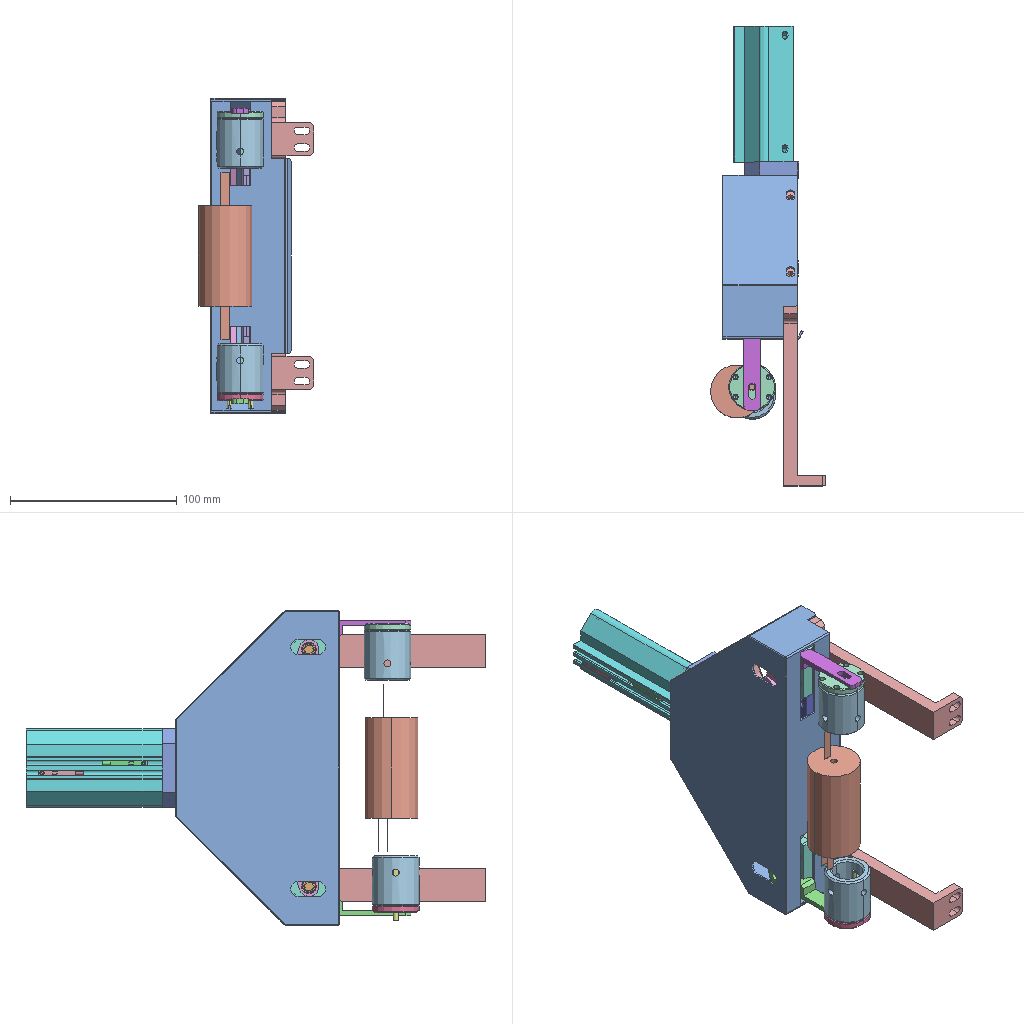Assembly | SolidWorks | 26 different items | 33 placed | box 69 x 276 x 189 mm
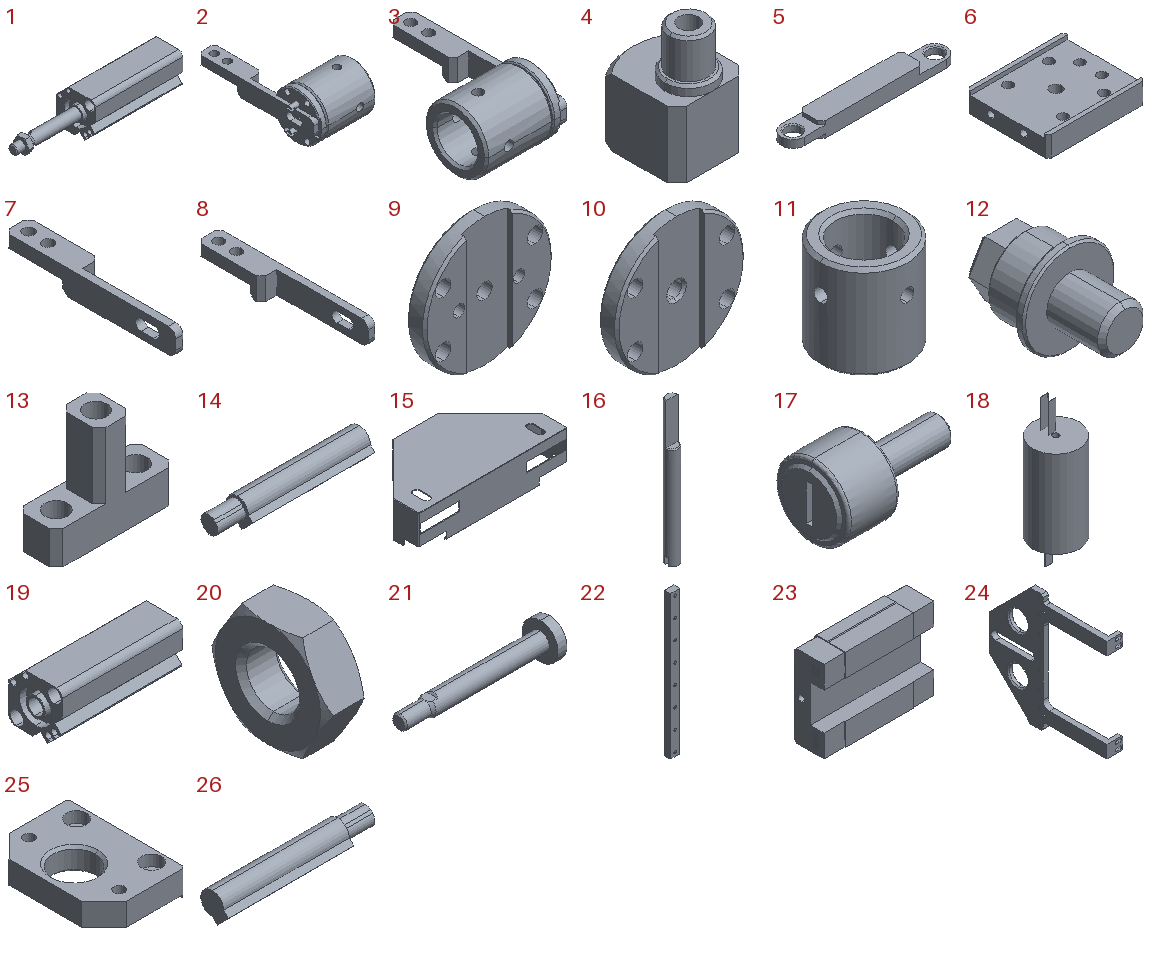Parts list (item | name | quantity | parent item | size | volume | features):
1 | (subassembly) | x1 | - | 140.657 x 36 x 36 mm | 68921 mm3 | features AEMSimFeature 1
2 | (subassembly) | x1 | - | 39 x 72.074 x 28 mm | 15051 mm3 | -
3 | (subassembly) | x1 | - | 36 x 70 x 28 mm | 14685 mm3 | -
4 | - | x1 | - | 15 x 17.5 x 24 mm | 3225 mm3 | features Chamfer 3, ICE 3, HoleWzd 2, Extrusion 1
5 | - | x2 | - | 87 x 12 x 8 mm | 6197 mm3 | features Chamfer 2, ICE 2, Extrusion 1
6 | - | x2 | - | 35.5 x 30 x 10.5 mm | 5956 mm3 | features HoleWzd 4, Chamfer 3, Cut 1, Extrusion 1, ICE 1
7 | - | x1 | in 2 | 10 x 70 x 10 mm | 2584 mm3 | features ICE 3, Chamfer 1, Extrusion 1, Fillet 1, HoleWzd 1
8 | - | x1 | in 3 | 10 x 70 x 10 mm | 2584 mm3 | features ICE 3, Chamfer 1, Extrusion 1, Fillet 1, HoleWzd 1
9 | - | x1 | in 2 | 28 x 5 x 28 mm | 2209 mm3 | features HoleWzd 3, Chamfer 2, ICE 2, Revolution 1
10 | - | x1 | in 3 | 28 x 5 x 28 mm | 2255 mm3 | features Chamfer 2, HoleWzd 2, ICE 2, Revolution 1
11 | - | x2 | in 2, 3 | 28 x 28 x 30 mm | 9846 mm3 | features HoleWzd 5, Chamfer 1, Extrusion 1
12 | - | x2 | - | 10 x 14 x 10 mm | 484.922 mm3 | features Chamfer 2, ICE 1, Revolution 1
13 | - | x2 | - | 18 x 6 x 15 mm | 590.913 mm3 | features Chamfer 2, HoleWzd 2, Extrusion 1, ICE 1
14 | - | x1 | in 1 | 27 x 4.828 x 4.828 mm | 354.995 mm3 | features BaseBody 1
15 | - | x1 | - | 189 x 98 x 48.5 mm | 32493 mm3 | features ICE 5, Chamfer 2, Fillet 2, BossThin 1, FlatPattern 1, MirrorPattern 1, SMBaseFlange 1, SheetMetal 1, Shell 1
16 | - | x2 | in 2 | 3 x 3 x 35 mm | 205.851 mm3 | features ICE 2, Chamfer 1, Extrusion 1
17 | - | x1 | - | 23 x 13 x 13 mm | 1507 mm3 | features ICE 1, Revolution 1
18 | - | x1 | - | 32 x 32 x 100 mm | 47531 mm3 | features ICE 2, Extrusion 1
19 | - | x1 | in 1 | 81.5 x 36 x 36 mm | 60391 mm3 | features BaseBody 1
20 | - | x1 | in 1 | 5 x 15.011 x 13 mm | 543.249 mm3 | features BaseBody 1
21 | - | x1 | in 1 | 83.5 x 20 x 20 mm | 7277 mm3 | features BaseBody 1
22 | - | x1 | - | 12 x 7.5 x 185 mm | 15537 mm3 | features Chamfer 1, Extrusion 1, HoleWzd 1, LPattern 1
23 | - | x2 | - | 35.4 x 10 x 27 mm | 7144 mm3 | features ICE 49, Chamfer 34, HoleWzd 16, RevCut 4, BaseBody 1
24 | - | x1 | - | 25 x 185 x 185 mm | 107483 mm3 | features HoleWzd 4, ICE 4, Chamfer 3, Fillet 2, Extrusion 1, MirrorPattern 1
25 | - | x1 | - | 32.5 x 47 x 10 mm | 10119 mm3 | features Chamfer 2, HoleWzd 2, ICE 2, Extrusion 1
26 | - | x1 | in 1 | 27 x 4.828 x 4.828 mm | 354.995 mm3 | features BaseBody 1
Mates (type | each side: item.copy, entity, surface, feature):
In the top assembly
DistanceDim | 18.1 plane | 24.1 face plane Boss-Extrude1
Coincident | 24.1 face plane Boss-Extrude1 | 22.1 face plane Boss-Extrude1
Width | 24.1 face plane Boss-Extrude1 | 24.1 face plane Boss-Extrude1 | 22.1 face plane Boss-Extrude1 | 22.1 face plane Boss-Extrude1
Coincident | 22.1 face plane Boss-Extrude1 | 23.1 face plane Cut-Revolve1
Coincident | 22.1 face plane Boss-Extrude1 | 23.2 face plane Cut-Revolve1
Coincident | 23.2 face plane Cut-Extrude41 | 22.1 face plane Boss-Extrude1
Coincident | 22.1 face plane Boss-Extrude1 | 23.1 face plane Cut-Extrude41
DistanceDim | 22.1 face plane Boss-Extrude1 | 24.1 face plane Boss-Extrude1
Coincident | 23.1 face plane Input3 | 6.1 face plane Cut-Extrude1
Coincident | 23.1 face plane Boss-Extrude1 | 6.1 face plane Cut-Extrude1
Coincident | 6.1 face plane Boss-Extrude1 | 23.1 face plane Input3
Coincident | 23.2 face plane Input3 | 6.2 face plane Cut-Extrude1
Coincident | 23.2 face plane Boss-Extrude1 | 6.2 face plane Cut-Extrude1
Coincident | 23.2 face plane Input3 | 6.2 face plane Boss-Extrude1
Concentric | 5.1 face cylinder Cut-Extrude2 | 5.2 face cylinder Cut-Extrude2
Concentric | 6.1 face cylinder M5 Tapped Hole1 | 5.1 face cylinder Cut-Extrude2
Concentric | 6.2 face cylinder M5 Tapped Hole1 | 5.2 face cylinder Cut-Extrude2
Coincident | 6.1 face plane Boss-Extrude1 | 12.1 face plane Revolve1
Concentric | 6.1 face cylinder M5 Tapped Hole1 | 12.1 face cylinder Revolve1
Concentric | 6.2 face cylinder M5 Tapped Hole1 | 12.2 face cylinder Revolve1
Coincident | 5.2 face plane Cut-Extrude3 | 12.2 face plane Revolve1
Coincident | 6.2 face plane Boss-Extrude1 | 12.2 face plane Revolve1
Coincident | 5.1 face plane Cut-Extrude3 | 12.1 face plane Revolve1
Concentric | 5.2 face cylinder Cut-Extrude2 | 17.1 face cylinder Revolve1
Tangent | 24.1 face plane Cut-Extrude5 | 17.1 face torus Revolve1
Concentric | 17.1 face cylinder Revolve1 | 4.1 face cylinder M5 Tapped Hole1
DistanceDim | 24.1 face plane Boss-Extrude1 | 17.1 face plane Revolve1
Coincident | 5.1 face plane Boss-Extrude1 | 4.1 face plane Boss-Extrude2
Parallel | 24.1 face plane Boss-Extrude1 | 4.1 face plane Cut-Extrude2
Width | 24.1 face plane Boss-Extrude1 | 24.1 face plane Boss-Extrude1 | 18.1 face plane Boss-Extrude1 | 18.1 face plane Boss-Extrude1
Coincident | 6.2 face plane Cut-Extrude4 | 7.1 face plane Cut-Extrude2
Coincident | 6.2 face plane Boss-Extrude1 | 7.1 face plane Boss-Extrude1
Coincident | 6.2 face plane Boss-Extrude1 | 7.1 face plane Cut-Extrude2
Tangent | 4.1 face cylinder Boss-Extrude1 | 20.1 face plane Input1
Concentric | 4.1 face cylinder M8x1.0 Tapped Hole1 | 21.1 face cylinder Input1
Coincident | 24.1 face plane Boss-Extrude1 | 25.1 face plane Cut-Extrude1
Concentric | 24.1 face cylinder M4 Tapped Hole1 | 25.1 face cylinder CBORE for M4 Hex Socket Head Cap Screw1 | 2 times
Coincident | 19.1 face plane Input1 | 25.1 face plane Boss-Extrude1
Concentric | 19.1 face cylinder Input1 | 25.1 face cylinder M5 Tapped Hole1
Coincident | 6.1 face plane Cut-Extrude4 | 8.1 face plane Cut-Extrude2
Concentric | 8.1 face cylinder M4 Clearance Hole1 | 6.1 face cylinder M4 Tapped Hole3 | 2 times
Concentric | 6.2 face cylinder M3 Tapped Hole1 | 13.1 face cylinder M3 Clearance Hole1 | 2 times
Coincident | 6.2 face plane Boss-Extrude1 | 13.1 face plane Boss-Extrude2
Concentric | 6.1 face cylinder M3 Tapped Hole1 | 13.2 face cylinder M3 Clearance Hole1 | 2 times
Coincident | 6.1 face plane Boss-Extrude1 | 13.2 face plane Boss-Extrude2
Coincident | 24.1 face plane Boss-Extrude1 | 15.1 face plane Shell1
Coincident | 24.1 face plane Boss-Extrude1 | 15.1 face plane Base-Flange1
Width | 15.1 face plane Base-Flange1 | 15.1 face plane Base-Flange1 | 24.1 face plane Cut-Extrude6 | 24.1 face plane Cut-Extrude6
In subassembly 2
Coincident | 7.2 face plane Cut-Extrude1 | 9.1 face plane Cut-Extrude3
Coincident | 7.2 face plane Boss-Extrude1 | 9.1 face plane Cut-Extrude3
Coincident | 9.1 face plane Cut-Extrude2 | 11.1 face plane Boss-Extrude1
Concentric | 9.1 face cylinder M3 Clearance Hole1 | 11.1 face cylinder M3 Tapped Hole1 | 2 times
LimitDistanceDim | 11.1 plane | 7.2 face plane Boss-Extrude1
Concentric | 9.1 face cylinder M3 Tapped Hole1 | 16.1 face cylinder Boss-Extrude1
DistanceDim | 9.1 face plane Revolve1 | 16.1 face plane Boss-Extrude1
Parallel | 7.2 face plane Boss-Extrude1 | 16.1 face plane Cut-Extrude1
Concentric | 9.1 face cylinder M3 Tapped Hole1 | 16.2 face cylinder Boss-Extrude1
Coincident | 16.1 face plane Boss-Extrude1 | 16.2 face plane Boss-Extrude1
Parallel | 16.1 face plane Cut-Extrude1 | 16.2 face plane Cut-Extrude1
In subassembly 3
Coincident | 8.2 face plane Cut-Extrude1 | 10.1 face plane Cut-Extrude3
Coincident | 8.2 face plane Boss-Extrude1 | 10.1 face plane Cut-Extrude3
LimitDistanceDim | 10.1 plane | 8.2 face plane Boss-Extrude1
Coincident | 10.1 face plane Cut-Extrude2 | 11.1 face plane Boss-Extrude1
Concentric | 10.1 face cylinder M3 Clearance Hole1 | 11.1 face cylinder M3 Tapped Hole1 | 2 times
In subassembly 1
Concentric | 19.2 face cylinder Input1 | 21.2 face cylinder Input1
LimitDistanceDim | 21.2 face plane Input1 | 19.2 face plane Input1
DistanceDim | 20.2 face plane Input1 | 21.2 face plane Input1
Concentric | 21.2 face cylinder Input1 | 20.2 face cylinder Input1
DistanceDim | 14.1 face plane Input1 | 19.2 face plane Input1
Concentric | 19.2 face cylinder Input1 | 14.1 face cylinder Input1
Parallel | 19.2 face plane Input1 | 14.1 face plane Input1
DistanceDim | 26.1 face plane Input1 | 19.2 face plane Input1
Concentric | 19.2 face cylinder Input1 | 26.1 face cylinder Input1
Parallel | 19.2 face plane Input1 | 26.1 face plane Input1